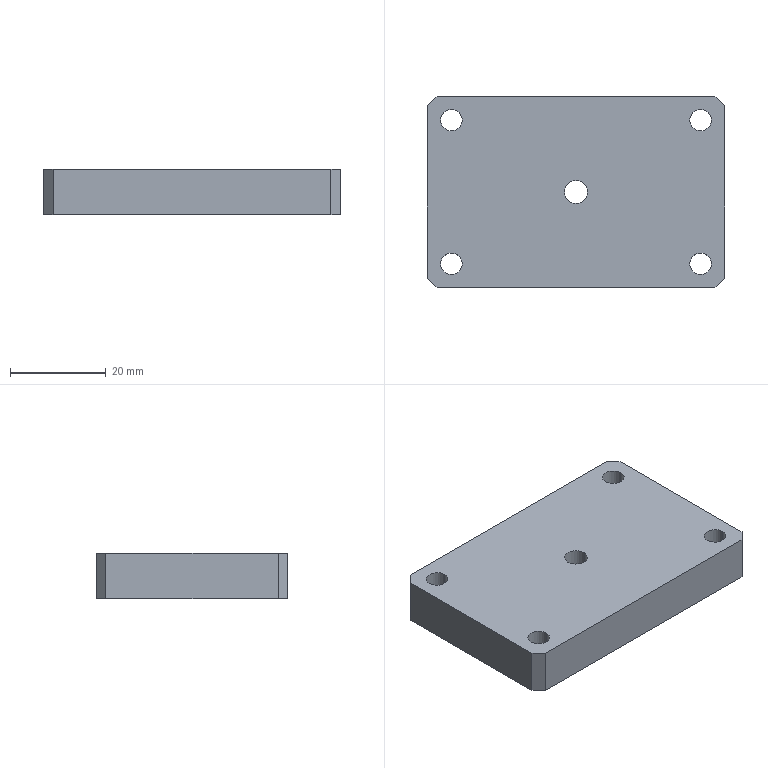Part | STEP file | 01-04 cylinder pad block | 1 solid | 23 faces | box 62 x 40 x 9.5 mm | volume 22560 mm3 | cylinder 12 | plane 11 | commonest cylinder face diameters 4.5 x8 4.8 x2 8 x2
STEP:
#1=CARTESIAN_POINT('',(23.75,15.,0.));
#2=VERTEX_POINT('',#1);
#3=CARTESIAN_POINT('',(28.25,15.,0.));
#4=VERTEX_POINT('',#3);
#5=CARTESIAN_POINT('',(26.,15.,0.));
#6=DIRECTION('',(0.,0.,1.));
#7=DIRECTION('',(1.,0.,0.));
#8=AXIS2_PLACEMENT_3D('',#5,#6,#7);
#9=CIRCLE('',#8,2.25);
#10=EDGE_CURVE('',#2,#4,#9,.T.);
#11=ORIENTED_EDGE('',*,*,#10,.F.);
#12=CARTESIAN_POINT('',(23.75,15.,9.5));
#13=VERTEX_POINT('',#12);
#14=CARTESIAN_POINT('',(23.75,15.,9.5));
#15=DIRECTION('',(0.,0.,1.));
#16=VECTOR('',#15,1000.);
#17=LINE('',#14,#16);
#18=EDGE_CURVE('',#2,#13,#17,.T.);
#19=ORIENTED_EDGE('',*,*,#18,.T.);
#20=CARTESIAN_POINT('',(28.25,15.,9.5));
#21=VERTEX_POINT('',#20);
#22=CARTESIAN_POINT('',(26.,15.,9.5));
#23=DIRECTION('',(0.,0.,1.));
#24=DIRECTION('',(1.,0.,0.));
#25=AXIS2_PLACEMENT_3D('',#22,#23,#24);
#26=CIRCLE('',#25,2.25);
#27=EDGE_CURVE('',#13,#21,#26,.T.);
#28=ORIENTED_EDGE('',*,*,#27,.T.);
#29=CARTESIAN_POINT('',(28.25,15.,9.5));
#30=DIRECTION('',(0.,0.,1.));
#31=VECTOR('',#30,1000.);
#32=LINE('',#29,#31);
#33=EDGE_CURVE('',#4,#21,#32,.T.);
#34=ORIENTED_EDGE('',*,*,#33,.F.);
#35=EDGE_LOOP('',(#11,#19,#28,#34));
#36=FACE_OUTER_BOUND('',#35,.T.);
#37=CARTESIAN_POINT('',(26.,15.,9.5));
#38=DIRECTION('',(0.,0.,1.));
#39=DIRECTION('',(1.,0.,0.));
#40=AXIS2_PLACEMENT_3D('',#37,#38,#39);
#41=CYLINDRICAL_SURFACE('',#40,2.25);
#42=ADVANCED_FACE('',(#36),#41,.F.);
#43=CARTESIAN_POINT('',(23.75,-15.,0.));
#44=VERTEX_POINT('',#43);
#45=CARTESIAN_POINT('',(28.25,-15.,0.));
#46=VERTEX_POINT('',#45);
#47=CARTESIAN_POINT('',(26.,-15.,0.));
#48=DIRECTION('',(0.,0.,1.));
#49=DIRECTION('',(1.,0.,0.));
#50=AXIS2_PLACEMENT_3D('',#47,#48,#49);
#51=CIRCLE('',#50,2.25);
#52=EDGE_CURVE('',#44,#46,#51,.T.);
#53=ORIENTED_EDGE('',*,*,#52,.F.);
#54=CARTESIAN_POINT('',(23.75,-15.,9.5));
#55=VERTEX_POINT('',#54);
#56=CARTESIAN_POINT('',(23.75,-15.,9.5));
#57=DIRECTION('',(0.,0.,1.));
#58=VECTOR('',#57,1000.);
#59=LINE('',#56,#58);
#60=EDGE_CURVE('',#44,#55,#59,.T.);
#61=ORIENTED_EDGE('',*,*,#60,.T.);
#62=CARTESIAN_POINT('',(28.25,-15.,9.5));
#63=VERTEX_POINT('',#62);
#64=CARTESIAN_POINT('',(26.,-15.,9.5));
#65=DIRECTION('',(0.,0.,1.));
#66=DIRECTION('',(1.,0.,0.));
#67=AXIS2_PLACEMENT_3D('',#64,#65,#66);
#68=CIRCLE('',#67,2.25);
#69=EDGE_CURVE('',#55,#63,#68,.T.);
#70=ORIENTED_EDGE('',*,*,#69,.T.);
#71=CARTESIAN_POINT('',(28.25,-15.,9.5));
#72=DIRECTION('',(0.,0.,1.));
#73=VECTOR('',#72,1000.);
#74=LINE('',#71,#73);
#75=EDGE_CURVE('',#46,#63,#74,.T.);
#76=ORIENTED_EDGE('',*,*,#75,.F.);
#77=EDGE_LOOP('',(#53,#61,#70,#76));
#78=FACE_OUTER_BOUND('',#77,.T.);
#79=CARTESIAN_POINT('',(26.,-15.,9.5));
#80=DIRECTION('',(0.,0.,1.));
#81=DIRECTION('',(1.,0.,0.));
#82=AXIS2_PLACEMENT_3D('',#79,#80,#81);
#83=CYLINDRICAL_SURFACE('',#82,2.25);
#84=ADVANCED_FACE('',(#78),#83,.F.);
#85=CARTESIAN_POINT('',(-28.25,-15.,0.));
#86=VERTEX_POINT('',#85);
#87=CARTESIAN_POINT('',(-23.75,-15.,0.));
#88=VERTEX_POINT('',#87);
#89=CARTESIAN_POINT('',(-26.,-15.,0.));
#90=DIRECTION('',(0.,0.,1.));
#91=DIRECTION('',(1.,0.,0.));
#92=AXIS2_PLACEMENT_3D('',#89,#90,#91);
#93=CIRCLE('',#92,2.25);
#94=EDGE_CURVE('',#86,#88,#93,.T.);
#95=ORIENTED_EDGE('',*,*,#94,.F.);
#96=CARTESIAN_POINT('',(-28.25,-15.,9.5));
#97=VERTEX_POINT('',#96);
#98=CARTESIAN_POINT('',(-28.25,-15.,9.5));
#99=DIRECTION('',(0.,0.,1.));
#100=VECTOR('',#99,1000.);
#101=LINE('',#98,#100);
#102=EDGE_CURVE('',#86,#97,#101,.T.);
#103=ORIENTED_EDGE('',*,*,#102,.T.);
#104=CARTESIAN_POINT('',(-23.75,-15.,9.5));
#105=VERTEX_POINT('',#104);
#106=CARTESIAN_POINT('',(-26.,-15.,9.5));
#107=DIRECTION('',(0.,0.,1.));
#108=DIRECTION('',(1.,0.,0.));
#109=AXIS2_PLACEMENT_3D('',#106,#107,#108);
#110=CIRCLE('',#109,2.25);
#111=EDGE_CURVE('',#97,#105,#110,.T.);
#112=ORIENTED_EDGE('',*,*,#111,.T.);
#113=CARTESIAN_POINT('',(-23.75,-15.,9.5));
#114=DIRECTION('',(0.,0.,1.));
#115=VECTOR('',#114,1000.);
#116=LINE('',#113,#115);
#117=EDGE_CURVE('',#88,#105,#116,.T.);
#118=ORIENTED_EDGE('',*,*,#117,.F.);
#119=EDGE_LOOP('',(#95,#103,#112,#118));
#120=FACE_OUTER_BOUND('',#119,.T.);
#121=CARTESIAN_POINT('',(-26.,-15.,9.5));
#122=DIRECTION('',(0.,0.,1.));
#123=DIRECTION('',(1.,0.,0.));
#124=AXIS2_PLACEMENT_3D('',#121,#122,#123);
#125=CYLINDRICAL_SURFACE('',#124,2.25);
#126=ADVANCED_FACE('',(#120),#125,.F.);
#127=CARTESIAN_POINT('',(-28.25,15.,0.));
#128=VERTEX_POINT('',#127);
#129=CARTESIAN_POINT('',(-23.75,15.,0.));
#130=VERTEX_POINT('',#129);
#131=CARTESIAN_POINT('',(-26.,15.,0.));
#132=DIRECTION('',(0.,0.,1.));
#133=DIRECTION('',(1.,0.,0.));
#134=AXIS2_PLACEMENT_3D('',#131,#132,#133);
#135=CIRCLE('',#134,2.25);
#136=EDGE_CURVE('',#128,#130,#135,.T.);
#137=ORIENTED_EDGE('',*,*,#136,.F.);
#138=CARTESIAN_POINT('',(-28.25,15.,9.5));
#139=VERTEX_POINT('',#138);
#140=CARTESIAN_POINT('',(-28.25,15.,9.5));
#141=DIRECTION('',(0.,0.,1.));
#142=VECTOR('',#141,1000.);
#143=LINE('',#140,#142);
#144=EDGE_CURVE('',#128,#139,#143,.T.);
#145=ORIENTED_EDGE('',*,*,#144,.T.);
#146=CARTESIAN_POINT('',(-23.75,15.,9.5));
#147=VERTEX_POINT('',#146);
#148=CARTESIAN_POINT('',(-26.,15.,9.5));
#149=DIRECTION('',(0.,0.,1.));
#150=DIRECTION('',(1.,0.,0.));
#151=AXIS2_PLACEMENT_3D('',#148,#149,#150);
#152=CIRCLE('',#151,2.25);
#153=EDGE_CURVE('',#139,#147,#152,.T.);
#154=ORIENTED_EDGE('',*,*,#153,.T.);
#155=CARTESIAN_POINT('',(-23.75,15.,9.5));
#156=DIRECTION('',(0.,0.,1.));
#157=VECTOR('',#156,1000.);
#158=LINE('',#155,#157);
#159=EDGE_CURVE('',#130,#147,#158,.T.);
#160=ORIENTED_EDGE('',*,*,#159,.F.);
#161=EDGE_LOOP('',(#137,#145,#154,#160));
#162=FACE_OUTER_BOUND('',#161,.T.);
#163=CARTESIAN_POINT('',(-26.,15.,9.5));
#164=DIRECTION('',(0.,0.,1.));
#165=DIRECTION('',(1.,0.,0.));
#166=AXIS2_PLACEMENT_3D('',#163,#164,#165);
#167=CYLINDRICAL_SURFACE('',#166,2.25);
#168=ADVANCED_FACE('',(#162),#167,.F.);
#169=CARTESIAN_POINT('',(4.,0.,4.6));
#170=VERTEX_POINT('',#169);
#171=CARTESIAN_POINT('',(-4.,0.,4.6));
#172=VERTEX_POINT('',#171);
#173=CARTESIAN_POINT('',(0.,0.,4.6));
#174=DIRECTION('',(0.,0.,-1.));
#175=DIRECTION('',(-1.,0.,0.));
#176=AXIS2_PLACEMENT_3D('',#173,#174,#175);
#177=CIRCLE('',#176,4.);
#178=EDGE_CURVE('',#170,#172,#177,.T.);
#179=ORIENTED_EDGE('',*,*,#178,.F.);
#180=CARTESIAN_POINT('',(4.,0.,0.));
#181=VERTEX_POINT('',#180);
#182=CARTESIAN_POINT('',(4.,0.,0.));
#183=DIRECTION('',(0.,0.,-1.));
#184=VECTOR('',#183,1000.);
#185=LINE('',#182,#184);
#186=EDGE_CURVE('',#170,#181,#185,.T.);
#187=ORIENTED_EDGE('',*,*,#186,.T.);
#188=CARTESIAN_POINT('',(-4.,0.,0.));
#189=VERTEX_POINT('',#188);
#190=CARTESIAN_POINT('',(0.,0.,0.));
#191=DIRECTION('',(0.,0.,-1.));
#192=DIRECTION('',(-1.,0.,0.));
#193=AXIS2_PLACEMENT_3D('',#190,#191,#192);
#194=CIRCLE('',#193,4.);
#195=EDGE_CURVE('',#181,#189,#194,.T.);
#196=ORIENTED_EDGE('',*,*,#195,.T.);
#197=CARTESIAN_POINT('',(-4.,0.,0.));
#198=DIRECTION('',(0.,0.,-1.));
#199=VECTOR('',#198,1000.);
#200=LINE('',#197,#199);
#201=EDGE_CURVE('',#172,#189,#200,.T.);
#202=ORIENTED_EDGE('',*,*,#201,.F.);
#203=EDGE_LOOP('',(#179,#187,#196,#202));
#204=FACE_OUTER_BOUND('',#203,.T.);
#205=CARTESIAN_POINT('',(0.,0.,0.));
#206=DIRECTION('',(0.,0.,-1.));
#207=DIRECTION('',(-1.,0.,0.));
#208=AXIS2_PLACEMENT_3D('',#205,#206,#207);
#209=CYLINDRICAL_SURFACE('',#208,4.);
#210=ADVANCED_FACE('',(#204),#209,.F.);
#211=CARTESIAN_POINT('',(2.4,0.,9.5));
#212=VERTEX_POINT('',#211);
#213=CARTESIAN_POINT('',(-2.4,0.,9.5));
#214=VERTEX_POINT('',#213);
#215=CARTESIAN_POINT('',(0.,0.,9.5));
#216=DIRECTION('',(0.,0.,-1.));
#217=DIRECTION('',(-1.,0.,0.));
#218=AXIS2_PLACEMENT_3D('',#215,#216,#217);
#219=CIRCLE('',#218,2.4);
#220=EDGE_CURVE('',#212,#214,#219,.T.);
#221=ORIENTED_EDGE('',*,*,#220,.F.);
#222=CARTESIAN_POINT('',(2.4,0.,4.6));
#223=VERTEX_POINT('',#222);
#224=CARTESIAN_POINT('',(2.4,0.,0.));
#225=DIRECTION('',(0.,0.,-1.));
#226=VECTOR('',#225,1000.);
#227=LINE('',#224,#226);
#228=EDGE_CURVE('',#212,#223,#227,.T.);
#229=ORIENTED_EDGE('',*,*,#228,.T.);
#230=CARTESIAN_POINT('',(-2.4,0.,4.6));
#231=VERTEX_POINT('',#230);
#232=CARTESIAN_POINT('',(0.,0.,4.6));
#233=DIRECTION('',(0.,0.,-1.));
#234=DIRECTION('',(-1.,0.,0.));
#235=AXIS2_PLACEMENT_3D('',#232,#233,#234);
#236=CIRCLE('',#235,2.4);
#237=EDGE_CURVE('',#223,#231,#236,.T.);
#238=ORIENTED_EDGE('',*,*,#237,.T.);
#239=CARTESIAN_POINT('',(-2.4,0.,0.));
#240=DIRECTION('',(0.,0.,-1.));
#241=VECTOR('',#240,1000.);
#242=LINE('',#239,#241);
#243=EDGE_CURVE('',#214,#231,#242,.T.);
#244=ORIENTED_EDGE('',*,*,#243,.F.);
#245=EDGE_LOOP('',(#221,#229,#238,#244));
#246=FACE_OUTER_BOUND('',#245,.T.);
#247=CARTESIAN_POINT('',(0.,0.,0.));
#248=DIRECTION('',(0.,0.,-1.));
#249=DIRECTION('',(-1.,0.,0.));
#250=AXIS2_PLACEMENT_3D('',#247,#248,#249);
#251=CYLINDRICAL_SURFACE('',#250,2.4);
#252=ADVANCED_FACE('',(#246),#251,.F.);
#253=CARTESIAN_POINT('',(31.,-18.,9.5));
#254=VERTEX_POINT('',#253);
#255=CARTESIAN_POINT('',(31.,18.,9.5));
#256=VERTEX_POINT('',#255);
#257=CARTESIAN_POINT('',(31.,20.,9.5));
#258=DIRECTION('',(0.,1.,0.));
#259=VECTOR('',#258,1000.);
#260=LINE('',#257,#259);
#261=EDGE_CURVE('',#254,#256,#260,.T.);
#262=ORIENTED_EDGE('',*,*,#261,.F.);
#263=CARTESIAN_POINT('',(31.,-18.,0.));
#264=VERTEX_POINT('',#263);
#265=CARTESIAN_POINT('',(31.,-18.,9.5));
#266=DIRECTION('',(0.,0.,-1.));
#267=VECTOR('',#266,1000.);
#268=LINE('',#265,#267);
#269=EDGE_CURVE('',#254,#264,#268,.T.);
#270=ORIENTED_EDGE('',*,*,#269,.T.);
#271=CARTESIAN_POINT('',(31.,18.,0.));
#272=VERTEX_POINT('',#271);
#273=CARTESIAN_POINT('',(31.,20.,0.));
#274=DIRECTION('',(0.,1.,0.));
#275=VECTOR('',#274,1000.);
#276=LINE('',#273,#275);
#277=EDGE_CURVE('',#264,#272,#276,.T.);
#278=ORIENTED_EDGE('',*,*,#277,.T.);
#279=CARTESIAN_POINT('',(31.,18.,9.5));
#280=DIRECTION('',(0.,0.,1.));
#281=VECTOR('',#280,1000.);
#282=LINE('',#279,#281);
#283=EDGE_CURVE('',#272,#256,#282,.T.);
#284=ORIENTED_EDGE('',*,*,#283,.T.);
#285=EDGE_LOOP('',(#262,#270,#278,#284));
#286=FACE_OUTER_BOUND('',#285,.T.);
#287=CARTESIAN_POINT('',(31.,20.,9.5));
#288=DIRECTION('',(-1.,0.,0.));
#289=DIRECTION('',(0.,-1.,0.));
#290=AXIS2_PLACEMENT_3D('',#287,#288,#289);
#291=PLANE('',#290);
#292=ADVANCED_FACE('',(#286),#291,.F.);
#293=CARTESIAN_POINT('',(29.,20.,9.5));
#294=VERTEX_POINT('',#293);
#295=CARTESIAN_POINT('',(-29.,20.,9.5));
#296=VERTEX_POINT('',#295);
#297=CARTESIAN_POINT('',(-31.,20.,9.5));
#298=DIRECTION('',(-1.,0.,0.));
#299=VECTOR('',#298,1000.);
#300=LINE('',#297,#299);
#301=EDGE_CURVE('',#294,#296,#300,.T.);
#302=ORIENTED_EDGE('',*,*,#301,.F.);
#303=CARTESIAN_POINT('',(29.,20.,0.));
#304=VERTEX_POINT('',#303);
#305=CARTESIAN_POINT('',(29.,20.,9.5));
#306=DIRECTION('',(0.,0.,-1.));
#307=VECTOR('',#306,1000.);
#308=LINE('',#305,#307);
#309=EDGE_CURVE('',#294,#304,#308,.T.);
#310=ORIENTED_EDGE('',*,*,#309,.T.);
#311=CARTESIAN_POINT('',(-29.,20.,0.));
#312=VERTEX_POINT('',#311);
#313=CARTESIAN_POINT('',(-31.,20.,0.));
#314=DIRECTION('',(-1.,0.,0.));
#315=VECTOR('',#314,1000.);
#316=LINE('',#313,#315);
#317=EDGE_CURVE('',#304,#312,#316,.T.);
#318=ORIENTED_EDGE('',*,*,#317,.T.);
#319=CARTESIAN_POINT('',(-29.,20.,9.5));
#320=DIRECTION('',(0.,0.,1.));
#321=VECTOR('',#320,1000.);
#322=LINE('',#319,#321);
#323=EDGE_CURVE('',#312,#296,#322,.T.);
#324=ORIENTED_EDGE('',*,*,#323,.T.);
#325=EDGE_LOOP('',(#302,#310,#318,#324));
#326=FACE_OUTER_BOUND('',#325,.T.);
#327=CARTESIAN_POINT('',(-31.,20.,9.5));
#328=DIRECTION('',(0.,-1.,0.));
#329=DIRECTION('',(0.,0.,-1.));
#330=AXIS2_PLACEMENT_3D('',#327,#328,#329);
#331=PLANE('',#330);
#332=ADVANCED_FACE('',(#326),#331,.F.);
#333=CARTESIAN_POINT('',(-31.,18.,9.5));
#334=VERTEX_POINT('',#333);
#335=CARTESIAN_POINT('',(-31.,-18.,9.5));
#336=VERTEX_POINT('',#335);
#337=CARTESIAN_POINT('',(-31.,20.,9.5));
#338=DIRECTION('',(0.,-1.,0.));
#339=VECTOR('',#338,1000.);
#340=LINE('',#337,#339);
#341=EDGE_CURVE('',#334,#336,#340,.T.);
#342=ORIENTED_EDGE('',*,*,#341,.F.);
#343=CARTESIAN_POINT('',(-31.,18.,0.));
#344=VERTEX_POINT('',#343);
#345=CARTESIAN_POINT('',(-31.,18.,9.5));
#346=DIRECTION('',(0.,0.,-1.));
#347=VECTOR('',#346,1000.);
#348=LINE('',#345,#347);
#349=EDGE_CURVE('',#334,#344,#348,.T.);
#350=ORIENTED_EDGE('',*,*,#349,.T.);
#351=CARTESIAN_POINT('',(-31.,-18.,0.));
#352=VERTEX_POINT('',#351);
#353=CARTESIAN_POINT('',(-31.,20.,0.));
#354=DIRECTION('',(0.,-1.,0.));
#355=VECTOR('',#354,1000.);
#356=LINE('',#353,#355);
#357=EDGE_CURVE('',#344,#352,#356,.T.);
#358=ORIENTED_EDGE('',*,*,#357,.T.);
#359=CARTESIAN_POINT('',(-31.,-18.,9.5));
#360=DIRECTION('',(0.,0.,1.));
#361=VECTOR('',#360,1000.);
#362=LINE('',#359,#361);
#363=EDGE_CURVE('',#352,#336,#362,.T.);
#364=ORIENTED_EDGE('',*,*,#363,.T.);
#365=EDGE_LOOP('',(#342,#350,#358,#364));
#366=FACE_OUTER_BOUND('',#365,.T.);
#367=CARTESIAN_POINT('',(-31.,20.,9.5));
#368=DIRECTION('',(1.,0.,0.));
#369=DIRECTION('',(0.,1.,0.));
#370=AXIS2_PLACEMENT_3D('',#367,#368,#369);
#371=PLANE('',#370);
#372=ADVANCED_FACE('',(#366),#371,.F.);
#373=CARTESIAN_POINT('',(-29.,-20.,0.));
#374=VERTEX_POINT('',#373);
#375=CARTESIAN_POINT('',(29.,-20.,0.));
#376=VERTEX_POINT('',#375);
#377=CARTESIAN_POINT('',(-31.,-20.,0.));
#378=DIRECTION('',(1.,0.,0.));
#379=VECTOR('',#378,1000.);
#380=LINE('',#377,#379);
#381=EDGE_CURVE('',#374,#376,#380,.T.);
#382=ORIENTED_EDGE('',*,*,#381,.T.);
#383=CARTESIAN_POINT('',(29.,-20.,9.5));
#384=VERTEX_POINT('',#383);
#385=CARTESIAN_POINT('',(29.,-20.,9.5));
#386=DIRECTION('',(0.,0.,1.));
#387=VECTOR('',#386,1000.);
#388=LINE('',#385,#387);
#389=EDGE_CURVE('',#376,#384,#388,.T.);
#390=ORIENTED_EDGE('',*,*,#389,.T.);
#391=CARTESIAN_POINT('',(-29.,-20.,9.5));
#392=VERTEX_POINT('',#391);
#393=CARTESIAN_POINT('',(-31.,-20.,9.5));
#394=DIRECTION('',(1.,0.,0.));
#395=VECTOR('',#394,1000.);
#396=LINE('',#393,#395);
#397=EDGE_CURVE('',#392,#384,#396,.T.);
#398=ORIENTED_EDGE('',*,*,#397,.F.);
#399=CARTESIAN_POINT('',(-29.,-20.,9.5));
#400=DIRECTION('',(0.,0.,-1.));
#401=VECTOR('',#400,1000.);
#402=LINE('',#399,#401);
#403=EDGE_CURVE('',#392,#374,#402,.T.);
#404=ORIENTED_EDGE('',*,*,#403,.T.);
#405=EDGE_LOOP('',(#382,#390,#398,#404));
#406=FACE_OUTER_BOUND('',#405,.T.);
#407=CARTESIAN_POINT('',(-31.,-20.,9.5));
#408=DIRECTION('',(0.,1.,0.));
#409=DIRECTION('',(0.,0.,1.));
#410=AXIS2_PLACEMENT_3D('',#407,#408,#409);
#411=PLANE('',#410);
#412=ADVANCED_FACE('',(#406),#411,.F.);
#413=CARTESIAN_POINT('',(26.,15.,9.5));
#414=DIRECTION('',(0.,0.,1.));
#415=DIRECTION('',(1.,0.,0.));
#416=AXIS2_PLACEMENT_3D('',#413,#414,#415);
#417=CIRCLE('',#416,2.25);
#418=EDGE_CURVE('',#21,#13,#417,.T.);
#419=ORIENTED_EDGE('',*,*,#418,.F.);
#420=ORIENTED_EDGE('',*,*,#27,.F.);
#421=EDGE_LOOP('',(#419,#420));
#422=FACE_BOUND('',#421,.T.);
#423=CARTESIAN_POINT('',(26.,-15.,9.5));
#424=DIRECTION('',(0.,0.,1.));
#425=DIRECTION('',(1.,0.,0.));
#426=AXIS2_PLACEMENT_3D('',#423,#424,#425);
#427=CIRCLE('',#426,2.25);
#428=EDGE_CURVE('',#63,#55,#427,.T.);
#429=ORIENTED_EDGE('',*,*,#428,.F.);
#430=ORIENTED_EDGE('',*,*,#69,.F.);
#431=EDGE_LOOP('',(#429,#430));
#432=FACE_BOUND('',#431,.T.);
#433=CARTESIAN_POINT('',(-26.,-15.,9.5));
#434=DIRECTION('',(0.,0.,1.));
#435=DIRECTION('',(1.,0.,0.));
#436=AXIS2_PLACEMENT_3D('',#433,#434,#435);
#437=CIRCLE('',#436,2.25);
#438=EDGE_CURVE('',#105,#97,#437,.T.);
#439=ORIENTED_EDGE('',*,*,#438,.F.);
#440=ORIENTED_EDGE('',*,*,#111,.F.);
#441=EDGE_LOOP('',(#439,#440));
#442=FACE_BOUND('',#441,.T.);
#443=CARTESIAN_POINT('',(-26.,15.,9.5));
#444=DIRECTION('',(0.,0.,1.));
#445=DIRECTION('',(1.,0.,0.));
#446=AXIS2_PLACEMENT_3D('',#443,#444,#445);
#447=CIRCLE('',#446,2.25);
#448=EDGE_CURVE('',#147,#139,#447,.T.);
#449=ORIENTED_EDGE('',*,*,#448,.F.);
#450=ORIENTED_EDGE('',*,*,#153,.F.);
#451=EDGE_LOOP('',(#449,#450));
#452=FACE_BOUND('',#451,.T.);
#453=CARTESIAN_POINT('',(0.,0.,9.5));
#454=DIRECTION('',(0.,0.,-1.));
#455=DIRECTION('',(-1.,0.,0.));
#456=AXIS2_PLACEMENT_3D('',#453,#454,#455);
#457=CIRCLE('',#456,2.4);
#458=EDGE_CURVE('',#214,#212,#457,.T.);
#459=ORIENTED_EDGE('',*,*,#458,.T.);
#460=ORIENTED_EDGE('',*,*,#220,.T.);
#461=EDGE_LOOP('',(#459,#460));
#462=FACE_BOUND('',#461,.T.);
#463=ORIENTED_EDGE('',*,*,#397,.T.);
#464=CARTESIAN_POINT('',(30.,-19.,9.5));
#465=DIRECTION('',(0.7071,0.7071,0.));
#466=VECTOR('',#465,1000.);
#467=LINE('',#464,#466);
#468=EDGE_CURVE('',#384,#254,#467,.T.);
#469=ORIENTED_EDGE('',*,*,#468,.T.);
#470=ORIENTED_EDGE('',*,*,#261,.T.);
#471=CARTESIAN_POINT('',(50.,-1.,9.5));
#472=DIRECTION('',(-0.7071,0.7071,0.));
#473=VECTOR('',#472,1000.);
#474=LINE('',#471,#473);
#475=EDGE_CURVE('',#256,#294,#474,.T.);
#476=ORIENTED_EDGE('',*,*,#475,.T.);
#477=ORIENTED_EDGE('',*,*,#301,.T.);
#478=CARTESIAN_POINT('',(-19.,30.,9.5));
#479=DIRECTION('',(-0.7071,-0.7071,0.));
#480=VECTOR('',#479,1000.);
#481=LINE('',#478,#480);
#482=EDGE_CURVE('',#296,#334,#481,.T.);
#483=ORIENTED_EDGE('',*,*,#482,.T.);
#484=ORIENTED_EDGE('',*,*,#341,.T.);
#485=CARTESIAN_POINT('',(1.,-50.,9.5));
#486=DIRECTION('',(0.7071,-0.7071,0.));
#487=VECTOR('',#486,1000.);
#488=LINE('',#485,#487);
#489=EDGE_CURVE('',#336,#392,#488,.T.);
#490=ORIENTED_EDGE('',*,*,#489,.T.);
#491=EDGE_LOOP('',(#463,#469,#470,#476,#477,#483,#484,#490));
#492=FACE_OUTER_BOUND('',#491,.T.);
#493=CARTESIAN_POINT('',(31.,-20.,9.5));
#494=DIRECTION('',(0.,0.,1.));
#495=DIRECTION('',(1.,0.,0.));
#496=AXIS2_PLACEMENT_3D('',#493,#494,#495);
#497=PLANE('',#496);
#498=ADVANCED_FACE('',(#422,#432,#442,#452,#462,#492),#497,.T.);
#499=CARTESIAN_POINT('',(26.,15.,0.));
#500=DIRECTION('',(0.,0.,1.));
#501=DIRECTION('',(1.,0.,0.));
#502=AXIS2_PLACEMENT_3D('',#499,#500,#501);
#503=CIRCLE('',#502,2.25);
#504=EDGE_CURVE('',#4,#2,#503,.T.);
#505=ORIENTED_EDGE('',*,*,#504,.T.);
#506=ORIENTED_EDGE('',*,*,#10,.T.);
#507=EDGE_LOOP('',(#505,#506));
#508=FACE_BOUND('',#507,.T.);
#509=CARTESIAN_POINT('',(26.,-15.,0.));
#510=DIRECTION('',(0.,0.,1.));
#511=DIRECTION('',(1.,0.,0.));
#512=AXIS2_PLACEMENT_3D('',#509,#510,#511);
#513=CIRCLE('',#512,2.25);
#514=EDGE_CURVE('',#46,#44,#513,.T.);
#515=ORIENTED_EDGE('',*,*,#514,.T.);
#516=ORIENTED_EDGE('',*,*,#52,.T.);
#517=EDGE_LOOP('',(#515,#516));
#518=FACE_BOUND('',#517,.T.);
#519=CARTESIAN_POINT('',(-26.,-15.,0.));
#520=DIRECTION('',(0.,0.,1.));
#521=DIRECTION('',(1.,0.,0.));
#522=AXIS2_PLACEMENT_3D('',#519,#520,#521);
#523=CIRCLE('',#522,2.25);
#524=EDGE_CURVE('',#88,#86,#523,.T.);
#525=ORIENTED_EDGE('',*,*,#524,.T.);
#526=ORIENTED_EDGE('',*,*,#94,.T.);
#527=EDGE_LOOP('',(#525,#526));
#528=FACE_BOUND('',#527,.T.);
#529=CARTESIAN_POINT('',(-26.,15.,0.));
#530=DIRECTION('',(0.,0.,1.));
#531=DIRECTION('',(1.,0.,0.));
#532=AXIS2_PLACEMENT_3D('',#529,#530,#531);
#533=CIRCLE('',#532,2.25);
#534=EDGE_CURVE('',#130,#128,#533,.T.);
#535=ORIENTED_EDGE('',*,*,#534,.T.);
#536=ORIENTED_EDGE('',*,*,#136,.T.);
#537=EDGE_LOOP('',(#535,#536));
#538=FACE_BOUND('',#537,.T.);
#539=CARTESIAN_POINT('',(0.,0.,0.));
#540=DIRECTION('',(0.,0.,-1.));
#541=DIRECTION('',(-1.,0.,0.));
#542=AXIS2_PLACEMENT_3D('',#539,#540,#541);
#543=CIRCLE('',#542,4.);
#544=EDGE_CURVE('',#189,#181,#543,.T.);
#545=ORIENTED_EDGE('',*,*,#544,.F.);
#546=ORIENTED_EDGE('',*,*,#195,.F.);
#547=EDGE_LOOP('',(#545,#546));
#548=FACE_BOUND('',#547,.T.);
#549=ORIENTED_EDGE('',*,*,#277,.F.);
#550=CARTESIAN_POINT('',(31.,-18.,0.));
#551=DIRECTION('',(-0.7071,-0.7071,0.));
#552=VECTOR('',#551,1000.);
#553=LINE('',#550,#552);
#554=EDGE_CURVE('',#264,#376,#553,.T.);
#555=ORIENTED_EDGE('',*,*,#554,.T.);
#556=ORIENTED_EDGE('',*,*,#381,.F.);
#557=CARTESIAN_POINT('',(-29.,-20.,0.));
#558=DIRECTION('',(-0.7071,0.7071,0.));
#559=VECTOR('',#558,1000.);
#560=LINE('',#557,#559);
#561=EDGE_CURVE('',#374,#352,#560,.T.);
#562=ORIENTED_EDGE('',*,*,#561,.T.);
#563=ORIENTED_EDGE('',*,*,#357,.F.);
#564=CARTESIAN_POINT('',(-31.,18.,0.));
#565=DIRECTION('',(0.7071,0.7071,0.));
#566=VECTOR('',#565,1000.);
#567=LINE('',#564,#566);
#568=EDGE_CURVE('',#344,#312,#567,.T.);
#569=ORIENTED_EDGE('',*,*,#568,.T.);
#570=ORIENTED_EDGE('',*,*,#317,.F.);
#571=CARTESIAN_POINT('',(29.,20.,0.));
#572=DIRECTION('',(0.7071,-0.7071,0.));
#573=VECTOR('',#572,1000.);
#574=LINE('',#571,#573);
#575=EDGE_CURVE('',#304,#272,#574,.T.);
#576=ORIENTED_EDGE('',*,*,#575,.T.);
#577=EDGE_LOOP('',(#549,#555,#556,#562,#563,#569,#570,#576));
#578=FACE_OUTER_BOUND('',#577,.T.);
#579=CARTESIAN_POINT('',(31.,-20.,0.));
#580=DIRECTION('',(0.,0.,1.));
#581=DIRECTION('',(1.,0.,0.));
#582=AXIS2_PLACEMENT_3D('',#579,#580,#581);
#583=PLANE('',#582);
#584=ADVANCED_FACE('',(#508,#518,#528,#538,#548,#578),#583,.F.);
#585=ORIENTED_EDGE('',*,*,#228,.F.);
#586=ORIENTED_EDGE('',*,*,#458,.F.);
#587=ORIENTED_EDGE('',*,*,#243,.T.);
#588=CARTESIAN_POINT('',(0.,0.,4.6));
#589=DIRECTION('',(0.,0.,-1.));
#590=DIRECTION('',(-1.,0.,0.));
#591=AXIS2_PLACEMENT_3D('',#588,#589,#590);
#592=CIRCLE('',#591,2.4);
#593=EDGE_CURVE('',#231,#223,#592,.T.);
#594=ORIENTED_EDGE('',*,*,#593,.T.);
#595=EDGE_LOOP('',(#585,#586,#587,#594));
#596=FACE_OUTER_BOUND('',#595,.T.);
#597=CARTESIAN_POINT('',(0.,0.,0.));
#598=DIRECTION('',(0.,0.,-1.));
#599=DIRECTION('',(-1.,0.,0.));
#600=AXIS2_PLACEMENT_3D('',#597,#598,#599);
#601=CYLINDRICAL_SURFACE('',#600,2.4);
#602=ADVANCED_FACE('',(#596),#601,.F.);
#603=ORIENTED_EDGE('',*,*,#593,.F.);
#604=ORIENTED_EDGE('',*,*,#237,.F.);
#605=EDGE_LOOP('',(#603,#604));
#606=FACE_BOUND('',#605,.T.);
#607=CARTESIAN_POINT('',(0.,0.,4.6));
#608=DIRECTION('',(0.,0.,-1.));
#609=DIRECTION('',(-1.,0.,0.));
#610=AXIS2_PLACEMENT_3D('',#607,#608,#609);
#611=CIRCLE('',#610,4.);
#612=EDGE_CURVE('',#172,#170,#611,.T.);
#613=ORIENTED_EDGE('',*,*,#612,.T.);
#614=ORIENTED_EDGE('',*,*,#178,.T.);
#615=EDGE_LOOP('',(#613,#614));
#616=FACE_OUTER_BOUND('',#615,.T.);
#617=CARTESIAN_POINT('',(2.4,0.,4.6));
#618=DIRECTION('',(0.,0.,1.));
#619=DIRECTION('',(1.,0.,0.));
#620=AXIS2_PLACEMENT_3D('',#617,#618,#619);
#621=PLANE('',#620);
#622=ADVANCED_FACE('',(#606,#616),#621,.F.);
#623=ORIENTED_EDGE('',*,*,#186,.F.);
#624=ORIENTED_EDGE('',*,*,#612,.F.);
#625=ORIENTED_EDGE('',*,*,#201,.T.);
#626=ORIENTED_EDGE('',*,*,#544,.T.);
#627=EDGE_LOOP('',(#623,#624,#625,#626));
#628=FACE_OUTER_BOUND('',#627,.T.);
#629=CARTESIAN_POINT('',(0.,0.,0.));
#630=DIRECTION('',(0.,0.,-1.));
#631=DIRECTION('',(-1.,0.,0.));
#632=AXIS2_PLACEMENT_3D('',#629,#630,#631);
#633=CYLINDRICAL_SURFACE('',#632,4.);
#634=ADVANCED_FACE('',(#628),#633,.F.);
#635=ORIENTED_EDGE('',*,*,#144,.F.);
#636=ORIENTED_EDGE('',*,*,#534,.F.);
#637=ORIENTED_EDGE('',*,*,#159,.T.);
#638=ORIENTED_EDGE('',*,*,#448,.T.);
#639=EDGE_LOOP('',(#635,#636,#637,#638));
#640=FACE_OUTER_BOUND('',#639,.T.);
#641=CARTESIAN_POINT('',(-26.,15.,9.5));
#642=DIRECTION('',(0.,0.,1.));
#643=DIRECTION('',(1.,0.,0.));
#644=AXIS2_PLACEMENT_3D('',#641,#642,#643);
#645=CYLINDRICAL_SURFACE('',#644,2.25);
#646=ADVANCED_FACE('',(#640),#645,.F.);
#647=ORIENTED_EDGE('',*,*,#102,.F.);
#648=ORIENTED_EDGE('',*,*,#524,.F.);
#649=ORIENTED_EDGE('',*,*,#117,.T.);
#650=ORIENTED_EDGE('',*,*,#438,.T.);
#651=EDGE_LOOP('',(#647,#648,#649,#650));
#652=FACE_OUTER_BOUND('',#651,.T.);
#653=CARTESIAN_POINT('',(-26.,-15.,9.5));
#654=DIRECTION('',(0.,0.,1.));
#655=DIRECTION('',(1.,0.,0.));
#656=AXIS2_PLACEMENT_3D('',#653,#654,#655);
#657=CYLINDRICAL_SURFACE('',#656,2.25);
#658=ADVANCED_FACE('',(#652),#657,.F.);
#659=ORIENTED_EDGE('',*,*,#60,.F.);
#660=ORIENTED_EDGE('',*,*,#514,.F.);
#661=ORIENTED_EDGE('',*,*,#75,.T.);
#662=ORIENTED_EDGE('',*,*,#428,.T.);
#663=EDGE_LOOP('',(#659,#660,#661,#662));
#664=FACE_OUTER_BOUND('',#663,.T.);
#665=CARTESIAN_POINT('',(26.,-15.,9.5));
#666=DIRECTION('',(0.,0.,1.));
#667=DIRECTION('',(1.,0.,0.));
#668=AXIS2_PLACEMENT_3D('',#665,#666,#667);
#669=CYLINDRICAL_SURFACE('',#668,2.25);
#670=ADVANCED_FACE('',(#664),#669,.F.);
#671=ORIENTED_EDGE('',*,*,#18,.F.);
#672=ORIENTED_EDGE('',*,*,#504,.F.);
#673=ORIENTED_EDGE('',*,*,#33,.T.);
#674=ORIENTED_EDGE('',*,*,#418,.T.);
#675=EDGE_LOOP('',(#671,#672,#673,#674));
#676=FACE_OUTER_BOUND('',#675,.T.);
#677=CARTESIAN_POINT('',(26.,15.,9.5));
#678=DIRECTION('',(0.,0.,1.));
#679=DIRECTION('',(1.,0.,0.));
#680=AXIS2_PLACEMENT_3D('',#677,#678,#679);
#681=CYLINDRICAL_SURFACE('',#680,2.25);
#682=ADVANCED_FACE('',(#676),#681,.F.);
#683=ORIENTED_EDGE('',*,*,#468,.F.);
#684=ORIENTED_EDGE('',*,*,#389,.F.);
#685=ORIENTED_EDGE('',*,*,#554,.F.);
#686=ORIENTED_EDGE('',*,*,#269,.F.);
#687=EDGE_LOOP('',(#683,#684,#685,#686));
#688=FACE_OUTER_BOUND('',#687,.T.);
#689=CARTESIAN_POINT('',(31.,-18.,9.5));
#690=DIRECTION('',(-0.7071,0.7071,0.));
#691=DIRECTION('',(-0.7071,-0.7071,0.));
#692=AXIS2_PLACEMENT_3D('',#689,#690,#691);
#693=PLANE('',#692);
#694=ADVANCED_FACE('',(#688),#693,.F.);
#695=ORIENTED_EDGE('',*,*,#475,.F.);
#696=ORIENTED_EDGE('',*,*,#283,.F.);
#697=ORIENTED_EDGE('',*,*,#575,.F.);
#698=ORIENTED_EDGE('',*,*,#309,.F.);
#699=EDGE_LOOP('',(#695,#696,#697,#698));
#700=FACE_OUTER_BOUND('',#699,.T.);
#701=CARTESIAN_POINT('',(29.,20.,9.5));
#702=DIRECTION('',(-0.7071,-0.7071,0.));
#703=DIRECTION('',(0.7071,-0.7071,0.));
#704=AXIS2_PLACEMENT_3D('',#701,#702,#703);
#705=PLANE('',#704);
#706=ADVANCED_FACE('',(#700),#705,.F.);
#707=ORIENTED_EDGE('',*,*,#482,.F.);
#708=ORIENTED_EDGE('',*,*,#323,.F.);
#709=ORIENTED_EDGE('',*,*,#568,.F.);
#710=ORIENTED_EDGE('',*,*,#349,.F.);
#711=EDGE_LOOP('',(#707,#708,#709,#710));
#712=FACE_OUTER_BOUND('',#711,.T.);
#713=CARTESIAN_POINT('',(-31.,18.,9.5));
#714=DIRECTION('',(0.7071,-0.7071,0.));
#715=DIRECTION('',(0.7071,0.7071,0.));
#716=AXIS2_PLACEMENT_3D('',#713,#714,#715);
#717=PLANE('',#716);
#718=ADVANCED_FACE('',(#712),#717,.F.);
#719=ORIENTED_EDGE('',*,*,#489,.F.);
#720=ORIENTED_EDGE('',*,*,#363,.F.);
#721=ORIENTED_EDGE('',*,*,#561,.F.);
#722=ORIENTED_EDGE('',*,*,#403,.F.);
#723=EDGE_LOOP('',(#719,#720,#721,#722));
#724=FACE_OUTER_BOUND('',#723,.T.);
#725=CARTESIAN_POINT('',(-29.,-20.,9.5));
#726=DIRECTION('',(0.7071,0.7071,0.));
#727=DIRECTION('',(-0.7071,0.7071,0.));
#728=AXIS2_PLACEMENT_3D('',#725,#726,#727);
#729=PLANE('',#728);
#730=ADVANCED_FACE('',(#724),#729,.F.);
#731=CLOSED_SHELL('',(#42,#84,#126,#168,#210,#252,#292,#332,#372,#412,#498,#584,#602,#622,#634,#646,#658,#670,#682,#694,#706,#718,#730));
#732=MANIFOLD_SOLID_BREP('',#731);
#733=CARTESIAN_POINT('',(0.,0.,0.));
#734=DIRECTION('',(0.,0.,1.));
#735=DIRECTION('',(1.,0.,0.));
#736=AXIS2_PLACEMENT_3D('',#733,#734,#735);
#737=(LENGTH_UNIT()NAMED_UNIT(*)SI_UNIT(.MILLI.,.METRE.));
#738=UNCERTAINTY_MEASURE_WITH_UNIT(LENGTH_MEASURE(0.00001),#737,'','');
#739=(NAMED_UNIT(*)PLANE_ANGLE_UNIT()SI_UNIT($,.RADIAN.));
#740=(NAMED_UNIT(*)SI_UNIT($,.STERADIAN.)SOLID_ANGLE_UNIT());
#741=(GEOMETRIC_REPRESENTATION_CONTEXT(3)GLOBAL_UNCERTAINTY_ASSIGNED_CONTEXT((#738))GLOBAL_UNIT_ASSIGNED_CONTEXT((#737,#739,#740))REPRESENTATION_CONTEXT('',''));
#742=ADVANCED_BREP_SHAPE_REPRESENTATION('',(#732,#736),#741);